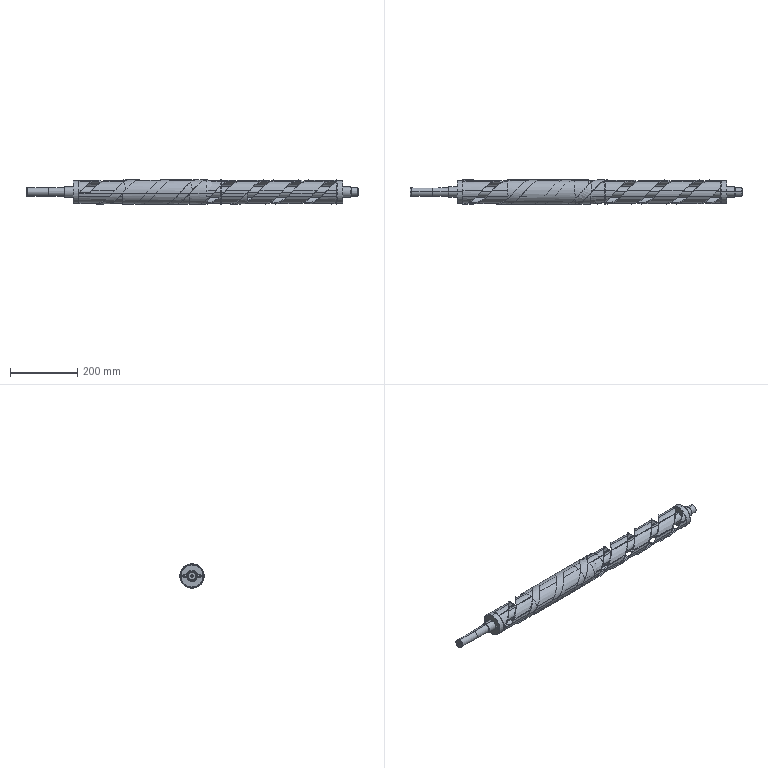Part | SolidWorks | features LayoutProfileFeature 1 | 5 solids | 271 faces | volume 3280765 mm3 | cylinder 129 | plane 101 | cone 22 | spline 19 | commonest cylinder face diameters 70 x42 65 x34 72 x14 8 x7 7 x4 7.5 x4